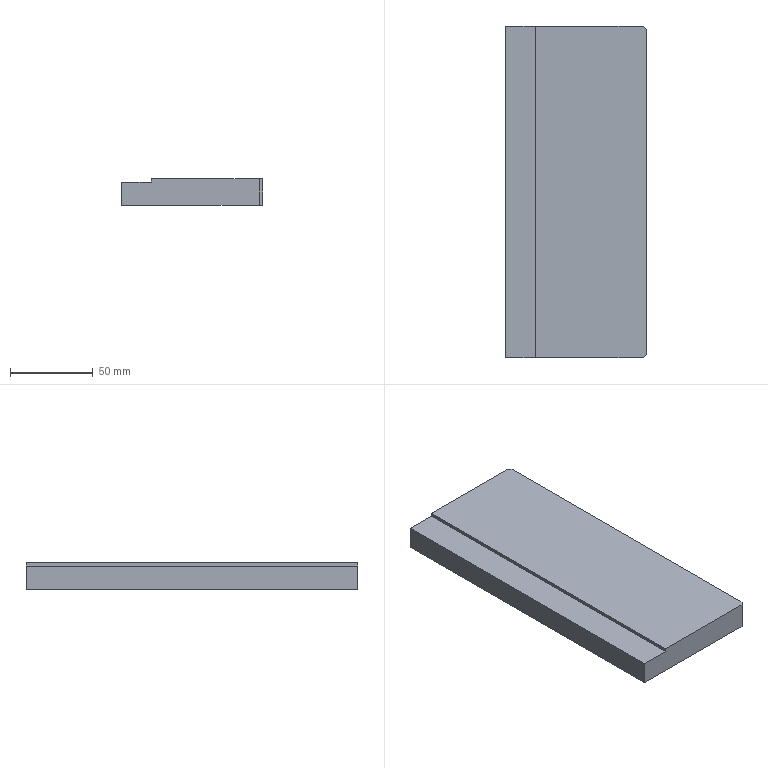Part | STEP file | PN_0036 | 1 solid | 10 faces | box 85 x 200 x 16 mm | volume 264736 mm3 | plane 10
STEP:
#1=CARTESIAN_POINT('',(0.,0.,0.));
#2=DIRECTION('',(0.,0.,1.));
#3=DIRECTION('',(1.,0.,0.));
#4=AXIS2_PLACEMENT_3D('',#1,#2,#3);
#5=CARTESIAN_POINT('',(-42.5,100.,14.));
#6=VERTEX_POINT('',#5);
#7=CARTESIAN_POINT('',(-42.5,-100.,14.));
#8=VERTEX_POINT('',#7);
#9=CARTESIAN_POINT('',(-42.5,100.,14.));
#10=DIRECTION('',(0.,-1.,0.));
#11=VECTOR('',#10,1.);
#12=LINE('',#9,#11);
#13=CARTESIAN_POINT('',(-42.5,100.,16.));
#14=DIRECTION('',(1.,0.,0.));
#15=DIRECTION('',(0.,1.,0.));
#16=AXIS2_PLACEMENT_3D('',#13,#14,#15);
#17=PLANE('',#16);
#18=CARTESIAN_POINT('',(0.,-2.));
#19=DIRECTION('',(-1.,0.));
#20=VECTOR('',#19,1.);
#21=LINE('',#18,#20);
#22=(GEOMETRIC_REPRESENTATION_CONTEXT(2)PARAMETRIC_REPRESENTATION_CONTEXT()REPRESENTATION_CONTEXT('',''));
#23=DEFINITIONAL_REPRESENTATION('',(#21),#22);
#24=PCURVE('',#17,#23);
#25=CARTESIAN_POINT('',(-42.5,-100.,14.));
#26=DIRECTION('',(0.,0.,1.));
#27=DIRECTION('',(1.,0.,0.));
#28=AXIS2_PLACEMENT_3D('',#25,#26,#27);
#29=PLANE('',#28);
#30=CARTESIAN_POINT('',(0.,200.));
#31=DIRECTION('',(0.,-1.));
#32=VECTOR('',#31,1.);
#33=LINE('',#30,#32);
#34=(GEOMETRIC_REPRESENTATION_CONTEXT(2)PARAMETRIC_REPRESENTATION_CONTEXT()REPRESENTATION_CONTEXT('',''));
#35=DEFINITIONAL_REPRESENTATION('',(#33),#34);
#36=PCURVE('',#29,#35);
#37=SURFACE_CURVE('',#12,(#24,#36),.PCURVE_S1.);
#38=EDGE_CURVE('',#6,#8,#37,.T.);
#39=ORIENTED_EDGE('',*,*,#38,.F.);
#40=CARTESIAN_POINT('',(-42.5,100.,0.));
#41=VERTEX_POINT('',#40);
#42=CARTESIAN_POINT('',(-42.5,100.,16.));
#43=DIRECTION('',(0.,0.,-1.));
#44=VECTOR('',#43,1.);
#45=LINE('',#42,#44);
#46=CARTESIAN_POINT('',(0.,0.));
#47=DIRECTION('',(0.,-1.));
#48=VECTOR('',#47,1.);
#49=LINE('',#46,#48);
#50=(GEOMETRIC_REPRESENTATION_CONTEXT(2)PARAMETRIC_REPRESENTATION_CONTEXT()REPRESENTATION_CONTEXT('',''));
#51=DEFINITIONAL_REPRESENTATION('',(#49),#50);
#52=PCURVE('',#17,#51);
#53=CARTESIAN_POINT('',(-42.5,100.,16.));
#54=DIRECTION('',(0.,-1.,0.));
#55=DIRECTION('',(0.,0.,-1.));
#56=AXIS2_PLACEMENT_3D('',#53,#54,#55);
#57=PLANE('',#56);
#58=CARTESIAN_POINT('',(0.,0.));
#59=DIRECTION('',(1.,0.));
#60=VECTOR('',#59,1.);
#61=LINE('',#58,#60);
#62=(GEOMETRIC_REPRESENTATION_CONTEXT(2)PARAMETRIC_REPRESENTATION_CONTEXT()REPRESENTATION_CONTEXT('',''));
#63=DEFINITIONAL_REPRESENTATION('',(#61),#62);
#64=PCURVE('',#57,#63);
#65=SURFACE_CURVE('',#45,(#52,#64),.PCURVE_S1.);
#66=EDGE_CURVE('',#6,#41,#65,.T.);
#67=ORIENTED_EDGE('',*,*,#66,.T.);
#68=CARTESIAN_POINT('',(-42.5,-100.,0.));
#69=VERTEX_POINT('',#68);
#70=CARTESIAN_POINT('',(-42.5,100.,0.));
#71=DIRECTION('',(0.,-1.,0.));
#72=VECTOR('',#71,1.);
#73=LINE('',#70,#72);
#74=CARTESIAN_POINT('',(0.,-16.));
#75=DIRECTION('',(-1.,0.));
#76=VECTOR('',#75,1.);
#77=LINE('',#74,#76);
#78=(GEOMETRIC_REPRESENTATION_CONTEXT(2)PARAMETRIC_REPRESENTATION_CONTEXT()REPRESENTATION_CONTEXT('',''));
#79=DEFINITIONAL_REPRESENTATION('',(#77),#78);
#80=PCURVE('',#17,#79);
#81=CARTESIAN_POINT('',(42.5,-100.,0.));
#82=DIRECTION('',(0.,0.,1.));
#83=DIRECTION('',(1.,0.,0.));
#84=AXIS2_PLACEMENT_3D('',#81,#82,#83);
#85=PLANE('',#84);
#86=CARTESIAN_POINT('',(-85.,200.));
#87=DIRECTION('',(0.,-1.));
#88=VECTOR('',#87,1.);
#89=LINE('',#86,#88);
#90=(GEOMETRIC_REPRESENTATION_CONTEXT(2)PARAMETRIC_REPRESENTATION_CONTEXT()REPRESENTATION_CONTEXT('',''));
#91=DEFINITIONAL_REPRESENTATION('',(#89),#90);
#92=PCURVE('',#85,#91);
#93=SURFACE_CURVE('',#73,(#80,#92),.PCURVE_S1.);
#94=EDGE_CURVE('',#41,#69,#93,.T.);
#95=ORIENTED_EDGE('',*,*,#94,.T.);
#96=CARTESIAN_POINT('',(-42.5,-100.,16.));
#97=DIRECTION('',(0.,0.,-1.));
#98=VECTOR('',#97,1.);
#99=LINE('',#96,#98);
#100=CARTESIAN_POINT('',(-200.,0.));
#101=DIRECTION('',(0.,-1.));
#102=VECTOR('',#101,1.);
#103=LINE('',#100,#102);
#104=(GEOMETRIC_REPRESENTATION_CONTEXT(2)PARAMETRIC_REPRESENTATION_CONTEXT()REPRESENTATION_CONTEXT('',''));
#105=DEFINITIONAL_REPRESENTATION('',(#103),#104);
#106=PCURVE('',#17,#105);
#107=CARTESIAN_POINT('',(-42.5,-100.,16.));
#108=DIRECTION('',(0.,1.,0.));
#109=DIRECTION('',(0.,0.,1.));
#110=AXIS2_PLACEMENT_3D('',#107,#108,#109);
#111=PLANE('',#110);
#112=CARTESIAN_POINT('',(0.,0.));
#113=DIRECTION('',(-1.,0.));
#114=VECTOR('',#113,1.);
#115=LINE('',#112,#114);
#116=(GEOMETRIC_REPRESENTATION_CONTEXT(2)PARAMETRIC_REPRESENTATION_CONTEXT()REPRESENTATION_CONTEXT('',''));
#117=DEFINITIONAL_REPRESENTATION('',(#115),#116);
#118=PCURVE('',#111,#117);
#119=SURFACE_CURVE('',#99,(#106,#118),.PCURVE_S1.);
#120=EDGE_CURVE('',#8,#69,#119,.T.);
#121=ORIENTED_EDGE('',*,*,#120,.F.);
#122=EDGE_LOOP('',(#39,#67,#95,#121));
#123=FACE_BOUND('',#122,.T.);
#124=ADVANCED_FACE('',(#123),#17,.F.);
#125=CARTESIAN_POINT('',(42.5,-98.,16.));
#126=VERTEX_POINT('',#125);
#127=CARTESIAN_POINT('',(42.5,98.,16.));
#128=VERTEX_POINT('',#127);
#129=CARTESIAN_POINT('',(42.5,100.,16.));
#130=DIRECTION('',(0.,1.,0.));
#131=VECTOR('',#130,1.);
#132=LINE('',#129,#131);
#133=CARTESIAN_POINT('',(42.5,100.,16.));
#134=DIRECTION('',(-1.,0.,0.));
#135=DIRECTION('',(0.,-1.,0.));
#136=AXIS2_PLACEMENT_3D('',#133,#134,#135);
#137=PLANE('',#136);
#138=CARTESIAN_POINT('',(0.,0.));
#139=DIRECTION('',(-1.,0.));
#140=VECTOR('',#139,1.);
#141=LINE('',#138,#140);
#142=(GEOMETRIC_REPRESENTATION_CONTEXT(2)PARAMETRIC_REPRESENTATION_CONTEXT()REPRESENTATION_CONTEXT('',''));
#143=DEFINITIONAL_REPRESENTATION('',(#141),#142);
#144=PCURVE('',#137,#143);
#145=CARTESIAN_POINT('',(42.5,-100.,16.));
#146=DIRECTION('',(0.,0.,1.));
#147=DIRECTION('',(1.,0.,0.));
#148=AXIS2_PLACEMENT_3D('',#145,#146,#147);
#149=PLANE('',#148);
#150=CARTESIAN_POINT('',(0.,200.));
#151=DIRECTION('',(0.,1.));
#152=VECTOR('',#151,1.);
#153=LINE('',#150,#152);
#154=(GEOMETRIC_REPRESENTATION_CONTEXT(2)PARAMETRIC_REPRESENTATION_CONTEXT()REPRESENTATION_CONTEXT('',''));
#155=DEFINITIONAL_REPRESENTATION('',(#153),#154);
#156=PCURVE('',#149,#155);
#157=SURFACE_CURVE('',#132,(#144,#156),.PCURVE_S1.);
#158=EDGE_CURVE('',#126,#128,#157,.T.);
#159=ORIENTED_EDGE('',*,*,#158,.F.);
#160=CARTESIAN_POINT('',(42.5,-98.,0.));
#161=VERTEX_POINT('',#160);
#162=CARTESIAN_POINT('',(42.5,-98.,16.));
#163=DIRECTION('',(0.,0.,-1.));
#164=VECTOR('',#163,1.);
#165=LINE('',#162,#164);
#166=CARTESIAN_POINT('',(198.,0.));
#167=DIRECTION('',(0.,-1.));
#168=VECTOR('',#167,1.);
#169=LINE('',#166,#168);
#170=(GEOMETRIC_REPRESENTATION_CONTEXT(2)PARAMETRIC_REPRESENTATION_CONTEXT()REPRESENTATION_CONTEXT('',''));
#171=DEFINITIONAL_REPRESENTATION('',(#169),#170);
#172=PCURVE('',#137,#171);
#173=CARTESIAN_POINT('',(42.5,-98.,16.));
#174=DIRECTION('',(-0.7071,0.7071,0.));
#175=DIRECTION('',(-0.7071,-0.7071,0.));
#176=AXIS2_PLACEMENT_3D('',#173,#174,#175);
#177=PLANE('',#176);
#178=CARTESIAN_POINT('',(0.,0.));
#179=DIRECTION('',(0.,-1.));
#180=VECTOR('',#179,1.);
#181=LINE('',#178,#180);
#182=(GEOMETRIC_REPRESENTATION_CONTEXT(2)PARAMETRIC_REPRESENTATION_CONTEXT()REPRESENTATION_CONTEXT('',''));
#183=DEFINITIONAL_REPRESENTATION('',(#181),#182);
#184=PCURVE('',#177,#183);
#185=SURFACE_CURVE('',#165,(#172,#184),.PCURVE_S1.);
#186=EDGE_CURVE('',#126,#161,#185,.T.);
#187=ORIENTED_EDGE('',*,*,#186,.T.);
#188=CARTESIAN_POINT('',(42.5,98.,0.));
#189=VERTEX_POINT('',#188);
#190=CARTESIAN_POINT('',(42.5,100.,0.));
#191=DIRECTION('',(0.,1.,0.));
#192=VECTOR('',#191,1.);
#193=LINE('',#190,#192);
#194=CARTESIAN_POINT('',(0.,-16.));
#195=DIRECTION('',(-1.,0.));
#196=VECTOR('',#195,1.);
#197=LINE('',#194,#196);
#198=(GEOMETRIC_REPRESENTATION_CONTEXT(2)PARAMETRIC_REPRESENTATION_CONTEXT()REPRESENTATION_CONTEXT('',''));
#199=DEFINITIONAL_REPRESENTATION('',(#197),#198);
#200=PCURVE('',#137,#199);
#201=CARTESIAN_POINT('',(0.,200.));
#202=DIRECTION('',(0.,1.));
#203=VECTOR('',#202,1.);
#204=LINE('',#201,#203);
#205=(GEOMETRIC_REPRESENTATION_CONTEXT(2)PARAMETRIC_REPRESENTATION_CONTEXT()REPRESENTATION_CONTEXT('',''));
#206=DEFINITIONAL_REPRESENTATION('',(#204),#205);
#207=PCURVE('',#85,#206);
#208=SURFACE_CURVE('',#193,(#200,#207),.PCURVE_S1.);
#209=EDGE_CURVE('',#161,#189,#208,.T.);
#210=ORIENTED_EDGE('',*,*,#209,.T.);
#211=CARTESIAN_POINT('',(42.5,98.,16.));
#212=DIRECTION('',(0.,0.,1.));
#213=VECTOR('',#212,1.);
#214=LINE('',#211,#213);
#215=CARTESIAN_POINT('',(2.,0.));
#216=DIRECTION('',(0.,1.));
#217=VECTOR('',#216,1.);
#218=LINE('',#215,#217);
#219=(GEOMETRIC_REPRESENTATION_CONTEXT(2)PARAMETRIC_REPRESENTATION_CONTEXT()REPRESENTATION_CONTEXT('',''));
#220=DEFINITIONAL_REPRESENTATION('',(#218),#219);
#221=PCURVE('',#137,#220);
#222=CARTESIAN_POINT('',(40.5,100.,16.));
#223=DIRECTION('',(-0.7071,-0.7071,0.));
#224=DIRECTION('',(0.7071,-0.7071,0.));
#225=AXIS2_PLACEMENT_3D('',#222,#223,#224);
#226=PLANE('',#225);
#227=CARTESIAN_POINT('',(2.828,0.));
#228=DIRECTION('',(0.,1.));
#229=VECTOR('',#228,1.);
#230=LINE('',#227,#229);
#231=(GEOMETRIC_REPRESENTATION_CONTEXT(2)PARAMETRIC_REPRESENTATION_CONTEXT()REPRESENTATION_CONTEXT('',''));
#232=DEFINITIONAL_REPRESENTATION('',(#230),#231);
#233=PCURVE('',#226,#232);
#234=SURFACE_CURVE('',#214,(#221,#233),.PCURVE_S1.);
#235=EDGE_CURVE('',#189,#128,#234,.T.);
#236=ORIENTED_EDGE('',*,*,#235,.T.);
#237=EDGE_LOOP('',(#159,#187,#210,#236));
#238=FACE_BOUND('',#237,.T.);
#239=ADVANCED_FACE('',(#238),#137,.F.);
#240=CARTESIAN_POINT('',(40.5,100.,16.));
#241=VERTEX_POINT('',#240);
#242=CARTESIAN_POINT('',(-24.5,100.,16.));
#243=VERTEX_POINT('',#242);
#244=CARTESIAN_POINT('',(-42.5,100.,16.));
#245=DIRECTION('',(-1.,0.,0.));
#246=VECTOR('',#245,1.);
#247=LINE('',#244,#246);
#248=CARTESIAN_POINT('',(0.,0.));
#249=DIRECTION('',(0.,-1.));
#250=VECTOR('',#249,1.);
#251=LINE('',#248,#250);
#252=(GEOMETRIC_REPRESENTATION_CONTEXT(2)PARAMETRIC_REPRESENTATION_CONTEXT()REPRESENTATION_CONTEXT('',''));
#253=DEFINITIONAL_REPRESENTATION('',(#251),#252);
#254=PCURVE('',#57,#253);
#255=CARTESIAN_POINT('',(-85.,200.));
#256=DIRECTION('',(-1.,0.));
#257=VECTOR('',#256,1.);
#258=LINE('',#255,#257);
#259=(GEOMETRIC_REPRESENTATION_CONTEXT(2)PARAMETRIC_REPRESENTATION_CONTEXT()REPRESENTATION_CONTEXT('',''));
#260=DEFINITIONAL_REPRESENTATION('',(#258),#259);
#261=PCURVE('',#149,#260);
#262=SURFACE_CURVE('',#247,(#254,#261),.PCURVE_S1.);
#263=EDGE_CURVE('',#241,#243,#262,.T.);
#264=ORIENTED_EDGE('',*,*,#263,.F.);
#265=CARTESIAN_POINT('',(40.5,100.,0.));
#266=VERTEX_POINT('',#265);
#267=CARTESIAN_POINT('',(40.5,100.,16.));
#268=DIRECTION('',(0.,0.,-1.));
#269=VECTOR('',#268,1.);
#270=LINE('',#267,#269);
#271=CARTESIAN_POINT('',(0.,83.));
#272=DIRECTION('',(1.,0.));
#273=VECTOR('',#272,1.);
#274=LINE('',#271,#273);
#275=(GEOMETRIC_REPRESENTATION_CONTEXT(2)PARAMETRIC_REPRESENTATION_CONTEXT()REPRESENTATION_CONTEXT('',''));
#276=DEFINITIONAL_REPRESENTATION('',(#274),#275);
#277=PCURVE('',#57,#276);
#278=CARTESIAN_POINT('',(0.,0.));
#279=DIRECTION('',(0.,-1.));
#280=VECTOR('',#279,1.);
#281=LINE('',#278,#280);
#282=(GEOMETRIC_REPRESENTATION_CONTEXT(2)PARAMETRIC_REPRESENTATION_CONTEXT()REPRESENTATION_CONTEXT('',''));
#283=DEFINITIONAL_REPRESENTATION('',(#281),#282);
#284=PCURVE('',#226,#283);
#285=SURFACE_CURVE('',#270,(#277,#284),.PCURVE_S1.);
#286=EDGE_CURVE('',#241,#266,#285,.T.);
#287=ORIENTED_EDGE('',*,*,#286,.T.);
#288=CARTESIAN_POINT('',(-42.5,100.,0.));
#289=DIRECTION('',(-1.,0.,0.));
#290=VECTOR('',#289,1.);
#291=LINE('',#288,#290);
#292=CARTESIAN_POINT('',(16.,0.));
#293=DIRECTION('',(0.,-1.));
#294=VECTOR('',#293,1.);
#295=LINE('',#292,#294);
#296=(GEOMETRIC_REPRESENTATION_CONTEXT(2)PARAMETRIC_REPRESENTATION_CONTEXT()REPRESENTATION_CONTEXT('',''));
#297=DEFINITIONAL_REPRESENTATION('',(#295),#296);
#298=PCURVE('',#57,#297);
#299=CARTESIAN_POINT('',(-85.,200.));
#300=DIRECTION('',(-1.,0.));
#301=VECTOR('',#300,1.);
#302=LINE('',#299,#301);
#303=(GEOMETRIC_REPRESENTATION_CONTEXT(2)PARAMETRIC_REPRESENTATION_CONTEXT()REPRESENTATION_CONTEXT('',''));
#304=DEFINITIONAL_REPRESENTATION('',(#302),#303);
#305=PCURVE('',#85,#304);
#306=SURFACE_CURVE('',#291,(#298,#305),.PCURVE_S1.);
#307=EDGE_CURVE('',#266,#41,#306,.T.);
#308=ORIENTED_EDGE('',*,*,#307,.T.);
#309=ORIENTED_EDGE('',*,*,#66,.F.);
#310=CARTESIAN_POINT('',(-24.5,100.,14.));
#311=VERTEX_POINT('',#310);
#312=CARTESIAN_POINT('',(-42.5,100.,14.));
#313=DIRECTION('',(-1.,0.,0.));
#314=VECTOR('',#313,1.);
#315=LINE('',#312,#314);
#316=CARTESIAN_POINT('',(2.,0.));
#317=DIRECTION('',(0.,-1.));
#318=VECTOR('',#317,1.);
#319=LINE('',#316,#318);
#320=(GEOMETRIC_REPRESENTATION_CONTEXT(2)PARAMETRIC_REPRESENTATION_CONTEXT()REPRESENTATION_CONTEXT('',''));
#321=DEFINITIONAL_REPRESENTATION('',(#319),#320);
#322=PCURVE('',#57,#321);
#323=CARTESIAN_POINT('',(0.,200.));
#324=DIRECTION('',(-1.,0.));
#325=VECTOR('',#324,1.);
#326=LINE('',#323,#325);
#327=(GEOMETRIC_REPRESENTATION_CONTEXT(2)PARAMETRIC_REPRESENTATION_CONTEXT()REPRESENTATION_CONTEXT('',''));
#328=DEFINITIONAL_REPRESENTATION('',(#326),#327);
#329=PCURVE('',#29,#328);
#330=SURFACE_CURVE('',#315,(#322,#329),.PCURVE_S1.);
#331=EDGE_CURVE('',#311,#6,#330,.T.);
#332=ORIENTED_EDGE('',*,*,#331,.F.);
#333=CARTESIAN_POINT('',(-24.5,100.,14.));
#334=DIRECTION('',(0.,0.,1.));
#335=VECTOR('',#334,1.);
#336=LINE('',#333,#335);
#337=CARTESIAN_POINT('',(2.,18.));
#338=DIRECTION('',(-1.,0.));
#339=VECTOR('',#338,1.);
#340=LINE('',#337,#339);
#341=(GEOMETRIC_REPRESENTATION_CONTEXT(2)PARAMETRIC_REPRESENTATION_CONTEXT()REPRESENTATION_CONTEXT('',''));
#342=DEFINITIONAL_REPRESENTATION('',(#340),#341);
#343=PCURVE('',#57,#342);
#344=CARTESIAN_POINT('',(-24.5,100.,14.));
#345=DIRECTION('',(1.,0.,0.));
#346=DIRECTION('',(0.,1.,0.));
#347=AXIS2_PLACEMENT_3D('',#344,#345,#346);
#348=PLANE('',#347);
#349=CARTESIAN_POINT('',(0.,0.));
#350=DIRECTION('',(0.,1.));
#351=VECTOR('',#350,1.);
#352=LINE('',#349,#351);
#353=(GEOMETRIC_REPRESENTATION_CONTEXT(2)PARAMETRIC_REPRESENTATION_CONTEXT()REPRESENTATION_CONTEXT('',''));
#354=DEFINITIONAL_REPRESENTATION('',(#352),#353);
#355=PCURVE('',#348,#354);
#356=SURFACE_CURVE('',#336,(#343,#355),.PCURVE_S1.);
#357=EDGE_CURVE('',#311,#243,#356,.T.);
#358=ORIENTED_EDGE('',*,*,#357,.T.);
#359=EDGE_LOOP('',(#264,#287,#308,#309,#332,#358));
#360=FACE_BOUND('',#359,.T.);
#361=ADVANCED_FACE('',(#360),#57,.F.);
#362=CARTESIAN_POINT('',(40.5,-100.,0.));
#363=VERTEX_POINT('',#362);
#364=CARTESIAN_POINT('',(-42.5,-100.,0.));
#365=DIRECTION('',(1.,0.,0.));
#366=VECTOR('',#365,1.);
#367=LINE('',#364,#366);
#368=CARTESIAN_POINT('',(-16.,0.));
#369=DIRECTION('',(0.,1.));
#370=VECTOR('',#369,1.);
#371=LINE('',#368,#370);
#372=(GEOMETRIC_REPRESENTATION_CONTEXT(2)PARAMETRIC_REPRESENTATION_CONTEXT()REPRESENTATION_CONTEXT('',''));
#373=DEFINITIONAL_REPRESENTATION('',(#371),#372);
#374=PCURVE('',#111,#373);
#375=CARTESIAN_POINT('',(-85.,0.));
#376=DIRECTION('',(1.,0.));
#377=VECTOR('',#376,1.);
#378=LINE('',#375,#377);
#379=(GEOMETRIC_REPRESENTATION_CONTEXT(2)PARAMETRIC_REPRESENTATION_CONTEXT()REPRESENTATION_CONTEXT('',''));
#380=DEFINITIONAL_REPRESENTATION('',(#378),#379);
#381=PCURVE('',#85,#380);
#382=SURFACE_CURVE('',#367,(#374,#381),.PCURVE_S1.);
#383=EDGE_CURVE('',#69,#363,#382,.T.);
#384=ORIENTED_EDGE('',*,*,#383,.T.);
#385=CARTESIAN_POINT('',(40.5,-100.,16.));
#386=VERTEX_POINT('',#385);
#387=CARTESIAN_POINT('',(40.5,-100.,16.));
#388=DIRECTION('',(0.,0.,1.));
#389=VECTOR('',#388,1.);
#390=LINE('',#387,#389);
#391=CARTESIAN_POINT('',(0.,83.));
#392=DIRECTION('',(1.,0.));
#393=VECTOR('',#392,1.);
#394=LINE('',#391,#393);
#395=(GEOMETRIC_REPRESENTATION_CONTEXT(2)PARAMETRIC_REPRESENTATION_CONTEXT()REPRESENTATION_CONTEXT('',''));
#396=DEFINITIONAL_REPRESENTATION('',(#394),#395);
#397=PCURVE('',#111,#396);
#398=CARTESIAN_POINT('',(2.828,0.));
#399=DIRECTION('',(0.,1.));
#400=VECTOR('',#399,1.);
#401=LINE('',#398,#400);
#402=(GEOMETRIC_REPRESENTATION_CONTEXT(2)PARAMETRIC_REPRESENTATION_CONTEXT()REPRESENTATION_CONTEXT('',''));
#403=DEFINITIONAL_REPRESENTATION('',(#401),#402);
#404=PCURVE('',#177,#403);
#405=SURFACE_CURVE('',#390,(#397,#404),.PCURVE_S1.);
#406=EDGE_CURVE('',#363,#386,#405,.T.);
#407=ORIENTED_EDGE('',*,*,#406,.T.);
#408=CARTESIAN_POINT('',(-24.5,-100.,16.));
#409=VERTEX_POINT('',#408);
#410=CARTESIAN_POINT('',(-42.5,-100.,16.));
#411=DIRECTION('',(1.,0.,0.));
#412=VECTOR('',#411,1.);
#413=LINE('',#410,#412);
#414=CARTESIAN_POINT('',(0.,0.));
#415=DIRECTION('',(0.,1.));
#416=VECTOR('',#415,1.);
#417=LINE('',#414,#416);
#418=(GEOMETRIC_REPRESENTATION_CONTEXT(2)PARAMETRIC_REPRESENTATION_CONTEXT()REPRESENTATION_CONTEXT('',''));
#419=DEFINITIONAL_REPRESENTATION('',(#417),#418);
#420=PCURVE('',#111,#419);
#421=CARTESIAN_POINT('',(-85.,0.));
#422=DIRECTION('',(1.,0.));
#423=VECTOR('',#422,1.);
#424=LINE('',#421,#423);
#425=(GEOMETRIC_REPRESENTATION_CONTEXT(2)PARAMETRIC_REPRESENTATION_CONTEXT()REPRESENTATION_CONTEXT('',''));
#426=DEFINITIONAL_REPRESENTATION('',(#424),#425);
#427=PCURVE('',#149,#426);
#428=SURFACE_CURVE('',#413,(#420,#427),.PCURVE_S1.);
#429=EDGE_CURVE('',#409,#386,#428,.T.);
#430=ORIENTED_EDGE('',*,*,#429,.F.);
#431=CARTESIAN_POINT('',(-24.5,-100.,14.));
#432=VERTEX_POINT('',#431);
#433=CARTESIAN_POINT('',(-24.5,-100.,14.));
#434=DIRECTION('',(0.,0.,1.));
#435=VECTOR('',#434,1.);
#436=LINE('',#433,#435);
#437=CARTESIAN_POINT('',(-2.,18.));
#438=DIRECTION('',(1.,0.));
#439=VECTOR('',#438,1.);
#440=LINE('',#437,#439);
#441=(GEOMETRIC_REPRESENTATION_CONTEXT(2)PARAMETRIC_REPRESENTATION_CONTEXT()REPRESENTATION_CONTEXT('',''));
#442=DEFINITIONAL_REPRESENTATION('',(#440),#441);
#443=PCURVE('',#111,#442);
#444=CARTESIAN_POINT('',(-200.,0.));
#445=DIRECTION('',(0.,1.));
#446=VECTOR('',#445,1.);
#447=LINE('',#444,#446);
#448=(GEOMETRIC_REPRESENTATION_CONTEXT(2)PARAMETRIC_REPRESENTATION_CONTEXT()REPRESENTATION_CONTEXT('',''));
#449=DEFINITIONAL_REPRESENTATION('',(#447),#448);
#450=PCURVE('',#348,#449);
#451=SURFACE_CURVE('',#436,(#443,#450),.PCURVE_S1.);
#452=EDGE_CURVE('',#432,#409,#451,.T.);
#453=ORIENTED_EDGE('',*,*,#452,.F.);
#454=CARTESIAN_POINT('',(-42.5,-100.,14.));
#455=DIRECTION('',(1.,0.,0.));
#456=VECTOR('',#455,1.);
#457=LINE('',#454,#456);
#458=CARTESIAN_POINT('',(-2.,0.));
#459=DIRECTION('',(0.,1.));
#460=VECTOR('',#459,1.);
#461=LINE('',#458,#460);
#462=(GEOMETRIC_REPRESENTATION_CONTEXT(2)PARAMETRIC_REPRESENTATION_CONTEXT()REPRESENTATION_CONTEXT('',''));
#463=DEFINITIONAL_REPRESENTATION('',(#461),#462);
#464=PCURVE('',#111,#463);
#465=CARTESIAN_POINT('',(0.,0.));
#466=DIRECTION('',(1.,0.));
#467=VECTOR('',#466,1.);
#468=LINE('',#465,#467);
#469=(GEOMETRIC_REPRESENTATION_CONTEXT(2)PARAMETRIC_REPRESENTATION_CONTEXT()REPRESENTATION_CONTEXT('',''));
#470=DEFINITIONAL_REPRESENTATION('',(#468),#469);
#471=PCURVE('',#29,#470);
#472=SURFACE_CURVE('',#457,(#464,#471),.PCURVE_S1.);
#473=EDGE_CURVE('',#8,#432,#472,.T.);
#474=ORIENTED_EDGE('',*,*,#473,.F.);
#475=ORIENTED_EDGE('',*,*,#120,.T.);
#476=EDGE_LOOP('',(#384,#407,#430,#453,#474,#475));
#477=FACE_BOUND('',#476,.T.);
#478=ADVANCED_FACE('',(#477),#111,.F.);
#479=ORIENTED_EDGE('',*,*,#429,.T.);
#480=CARTESIAN_POINT('',(41.5,-99.,16.));
#481=DIRECTION('',(0.7071,0.7071,0.));
#482=VECTOR('',#481,1.);
#483=LINE('',#480,#482);
#484=CARTESIAN_POINT('',(-1.,1.));
#485=DIRECTION('',(0.7071,0.7071));
#486=VECTOR('',#485,1.);
#487=LINE('',#484,#486);
#488=(GEOMETRIC_REPRESENTATION_CONTEXT(2)PARAMETRIC_REPRESENTATION_CONTEXT()REPRESENTATION_CONTEXT('',''));
#489=DEFINITIONAL_REPRESENTATION('',(#487),#488);
#490=PCURVE('',#149,#489);
#491=CARTESIAN_POINT('',(1.414,0.));
#492=DIRECTION('',(-1.,0.));
#493=VECTOR('',#492,1.);
#494=LINE('',#491,#493);
#495=(GEOMETRIC_REPRESENTATION_CONTEXT(2)PARAMETRIC_REPRESENTATION_CONTEXT()REPRESENTATION_CONTEXT('',''));
#496=DEFINITIONAL_REPRESENTATION('',(#494),#495);
#497=PCURVE('',#177,#496);
#498=SURFACE_CURVE('',#483,(#490,#497),.PCURVE_S1.);
#499=EDGE_CURVE('',#386,#126,#498,.T.);
#500=ORIENTED_EDGE('',*,*,#499,.T.);
#501=ORIENTED_EDGE('',*,*,#158,.T.);
#502=CARTESIAN_POINT('',(141.5,-1.,16.));
#503=DIRECTION('',(-0.7071,0.7071,0.));
#504=VECTOR('',#503,1.);
#505=LINE('',#502,#504);
#506=CARTESIAN_POINT('',(99.,99.));
#507=DIRECTION('',(-0.7071,0.7071));
#508=VECTOR('',#507,1.);
#509=LINE('',#506,#508);
#510=(GEOMETRIC_REPRESENTATION_CONTEXT(2)PARAMETRIC_REPRESENTATION_CONTEXT()REPRESENTATION_CONTEXT('',''));
#511=DEFINITIONAL_REPRESENTATION('',(#509),#510);
#512=PCURVE('',#149,#511);
#513=CARTESIAN_POINT('',(142.836,0.));
#514=DIRECTION('',(-1.,0.));
#515=VECTOR('',#514,1.);
#516=LINE('',#513,#515);
#517=(GEOMETRIC_REPRESENTATION_CONTEXT(2)PARAMETRIC_REPRESENTATION_CONTEXT()REPRESENTATION_CONTEXT('',''));
#518=DEFINITIONAL_REPRESENTATION('',(#516),#517);
#519=PCURVE('',#226,#518);
#520=SURFACE_CURVE('',#505,(#512,#519),.PCURVE_S1.);
#521=EDGE_CURVE('',#128,#241,#520,.T.);
#522=ORIENTED_EDGE('',*,*,#521,.T.);
#523=ORIENTED_EDGE('',*,*,#263,.T.);
#524=CARTESIAN_POINT('',(-24.5,100.,16.));
#525=DIRECTION('',(0.,1.,0.));
#526=VECTOR('',#525,1.);
#527=LINE('',#524,#526);
#528=CARTESIAN_POINT('',(-67.,200.));
#529=DIRECTION('',(0.,1.));
#530=VECTOR('',#529,1.);
#531=LINE('',#528,#530);
#532=(GEOMETRIC_REPRESENTATION_CONTEXT(2)PARAMETRIC_REPRESENTATION_CONTEXT()REPRESENTATION_CONTEXT('',''));
#533=DEFINITIONAL_REPRESENTATION('',(#531),#532);
#534=PCURVE('',#149,#533);
#535=CARTESIAN_POINT('',(0.,2.));
#536=DIRECTION('',(1.,0.));
#537=VECTOR('',#536,1.);
#538=LINE('',#535,#537);
#539=(GEOMETRIC_REPRESENTATION_CONTEXT(2)PARAMETRIC_REPRESENTATION_CONTEXT()REPRESENTATION_CONTEXT('',''));
#540=DEFINITIONAL_REPRESENTATION('',(#538),#539);
#541=PCURVE('',#348,#540);
#542=SURFACE_CURVE('',#527,(#534,#541),.PCURVE_S1.);
#543=EDGE_CURVE('',#409,#243,#542,.T.);
#544=ORIENTED_EDGE('',*,*,#543,.F.);
#545=EDGE_LOOP('',(#479,#500,#501,#522,#523,#544));
#546=FACE_BOUND('',#545,.T.);
#547=ADVANCED_FACE('',(#546),#149,.T.);
#548=ORIENTED_EDGE('',*,*,#209,.F.);
#549=CARTESIAN_POINT('',(42.5,-98.,0.));
#550=DIRECTION('',(-0.7071,-0.7071,0.));
#551=VECTOR('',#550,1.);
#552=LINE('',#549,#551);
#553=CARTESIAN_POINT('',(0.,2.));
#554=DIRECTION('',(-0.7071,-0.7071));
#555=VECTOR('',#554,1.);
#556=LINE('',#553,#555);
#557=(GEOMETRIC_REPRESENTATION_CONTEXT(2)PARAMETRIC_REPRESENTATION_CONTEXT()REPRESENTATION_CONTEXT('',''));
#558=DEFINITIONAL_REPRESENTATION('',(#556),#557);
#559=PCURVE('',#85,#558);
#560=CARTESIAN_POINT('',(0.,-16.));
#561=DIRECTION('',(1.,0.));
#562=VECTOR('',#561,1.);
#563=LINE('',#560,#562);
#564=(GEOMETRIC_REPRESENTATION_CONTEXT(2)PARAMETRIC_REPRESENTATION_CONTEXT()REPRESENTATION_CONTEXT('',''));
#565=DEFINITIONAL_REPRESENTATION('',(#563),#564);
#566=PCURVE('',#177,#565);
#567=SURFACE_CURVE('',#552,(#559,#566),.PCURVE_S1.);
#568=EDGE_CURVE('',#161,#363,#567,.T.);
#569=ORIENTED_EDGE('',*,*,#568,.T.);
#570=ORIENTED_EDGE('',*,*,#383,.F.);
#571=ORIENTED_EDGE('',*,*,#94,.F.);
#572=ORIENTED_EDGE('',*,*,#307,.F.);
#573=CARTESIAN_POINT('',(40.5,100.,0.));
#574=DIRECTION('',(0.7071,-0.7071,0.));
#575=VECTOR('',#574,1.);
#576=LINE('',#573,#575);
#577=CARTESIAN_POINT('',(-2.,200.));
#578=DIRECTION('',(0.7071,-0.7071));
#579=VECTOR('',#578,1.);
#580=LINE('',#577,#579);
#581=(GEOMETRIC_REPRESENTATION_CONTEXT(2)PARAMETRIC_REPRESENTATION_CONTEXT()REPRESENTATION_CONTEXT('',''));
#582=DEFINITIONAL_REPRESENTATION('',(#580),#581);
#583=PCURVE('',#85,#582);
#584=CARTESIAN_POINT('',(0.,-16.));
#585=DIRECTION('',(1.,0.));
#586=VECTOR('',#585,1.);
#587=LINE('',#584,#586);
#588=(GEOMETRIC_REPRESENTATION_CONTEXT(2)PARAMETRIC_REPRESENTATION_CONTEXT()REPRESENTATION_CONTEXT('',''));
#589=DEFINITIONAL_REPRESENTATION('',(#587),#588);
#590=PCURVE('',#226,#589);
#591=SURFACE_CURVE('',#576,(#583,#590),.PCURVE_S1.);
#592=EDGE_CURVE('',#266,#189,#591,.T.);
#593=ORIENTED_EDGE('',*,*,#592,.T.);
#594=EDGE_LOOP('',(#548,#569,#570,#571,#572,#593));
#595=FACE_BOUND('',#594,.T.);
#596=ADVANCED_FACE('',(#595),#85,.F.);
#597=ORIENTED_EDGE('',*,*,#543,.T.);
#598=ORIENTED_EDGE('',*,*,#357,.F.);
#599=CARTESIAN_POINT('',(-24.5,100.,14.));
#600=DIRECTION('',(0.,1.,0.));
#601=VECTOR('',#600,1.);
#602=LINE('',#599,#601);
#603=CARTESIAN_POINT('',(0.,0.));
#604=DIRECTION('',(1.,0.));
#605=VECTOR('',#604,1.);
#606=LINE('',#603,#605);
#607=(GEOMETRIC_REPRESENTATION_CONTEXT(2)PARAMETRIC_REPRESENTATION_CONTEXT()REPRESENTATION_CONTEXT('',''));
#608=DEFINITIONAL_REPRESENTATION('',(#606),#607);
#609=PCURVE('',#348,#608);
#610=CARTESIAN_POINT('',(18.,200.));
#611=DIRECTION('',(0.,1.));
#612=VECTOR('',#611,1.);
#613=LINE('',#610,#612);
#614=(GEOMETRIC_REPRESENTATION_CONTEXT(2)PARAMETRIC_REPRESENTATION_CONTEXT()REPRESENTATION_CONTEXT('',''));
#615=DEFINITIONAL_REPRESENTATION('',(#613),#614);
#616=PCURVE('',#29,#615);
#617=SURFACE_CURVE('',#602,(#609,#616),.PCURVE_S1.);
#618=EDGE_CURVE('',#432,#311,#617,.T.);
#619=ORIENTED_EDGE('',*,*,#618,.F.);
#620=ORIENTED_EDGE('',*,*,#452,.T.);
#621=EDGE_LOOP('',(#597,#598,#619,#620));
#622=FACE_BOUND('',#621,.T.);
#623=ADVANCED_FACE('',(#622),#348,.F.);
#624=ORIENTED_EDGE('',*,*,#38,.T.);
#625=ORIENTED_EDGE('',*,*,#473,.T.);
#626=ORIENTED_EDGE('',*,*,#618,.T.);
#627=ORIENTED_EDGE('',*,*,#331,.T.);
#628=EDGE_LOOP('',(#624,#625,#626,#627));
#629=FACE_BOUND('',#628,.T.);
#630=ADVANCED_FACE('',(#629),#29,.T.);
#631=ORIENTED_EDGE('',*,*,#499,.F.);
#632=ORIENTED_EDGE('',*,*,#406,.F.);
#633=ORIENTED_EDGE('',*,*,#568,.F.);
#634=ORIENTED_EDGE('',*,*,#186,.F.);
#635=EDGE_LOOP('',(#631,#632,#633,#634));
#636=FACE_BOUND('',#635,.T.);
#637=ADVANCED_FACE('',(#636),#177,.F.);
#638=ORIENTED_EDGE('',*,*,#521,.F.);
#639=ORIENTED_EDGE('',*,*,#235,.F.);
#640=ORIENTED_EDGE('',*,*,#592,.F.);
#641=ORIENTED_EDGE('',*,*,#286,.F.);
#642=EDGE_LOOP('',(#638,#639,#640,#641));
#643=FACE_BOUND('',#642,.T.);
#644=ADVANCED_FACE('',(#643),#226,.F.);
#645=CLOSED_SHELL('',(#124,#239,#361,#478,#547,#596,#623,#630,#637,#644));
#646=MANIFOLD_SOLID_BREP('',#645);
#647=(LENGTH_UNIT()NAMED_UNIT(*)SI_UNIT(.MILLI.,.METRE.));
#648=UNCERTAINTY_MEASURE_WITH_UNIT(LENGTH_MEASURE(0.0000001),#647,'','');
#649=(NAMED_UNIT(*)PLANE_ANGLE_UNIT()SI_UNIT($,.RADIAN.));
#650=(NAMED_UNIT(*)SI_UNIT($,.STERADIAN.)SOLID_ANGLE_UNIT());
#651=(GEOMETRIC_REPRESENTATION_CONTEXT(3)GLOBAL_UNCERTAINTY_ASSIGNED_CONTEXT((#648))GLOBAL_UNIT_ASSIGNED_CONTEXT((#647,#649,#650))REPRESENTATION_CONTEXT('',''));
#652=ADVANCED_BREP_SHAPE_REPRESENTATION('',(#4,#646),#651);